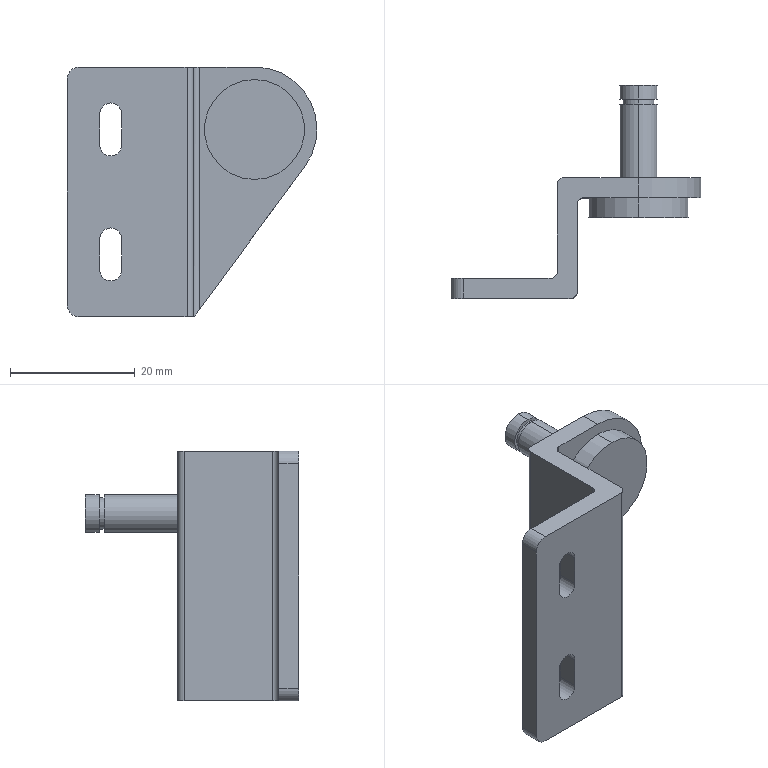Part | STEP file | Gas spring seat GSBR6B | 1 solid | 39 faces | box 40 x 34.1 x 40 mm | volume 7142 mm3 | cylinder 21 | plane 18 | commonest cylinder face diameters 3.5 x6 2 x4 6 x4 4 x2 5 x2 16 x2